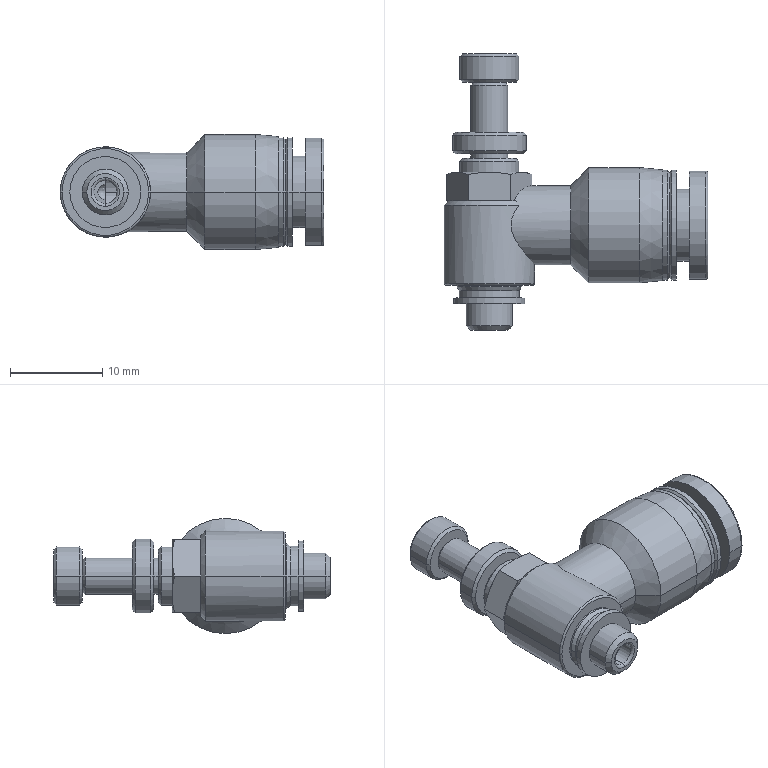Part | STEP file | 11-ASL5-M511 | 1 solid | 128 faces | box 28.6 x 30 x 12.5 mm | volume 2571 mm3 | plane 46 | cylinder 41 | cone 32 | torus 8 | sphere 1 | commonest cylinder face diameters 4 x6 6.4 x4 11.9 x4 2.5 x2 5 x2 6 x2